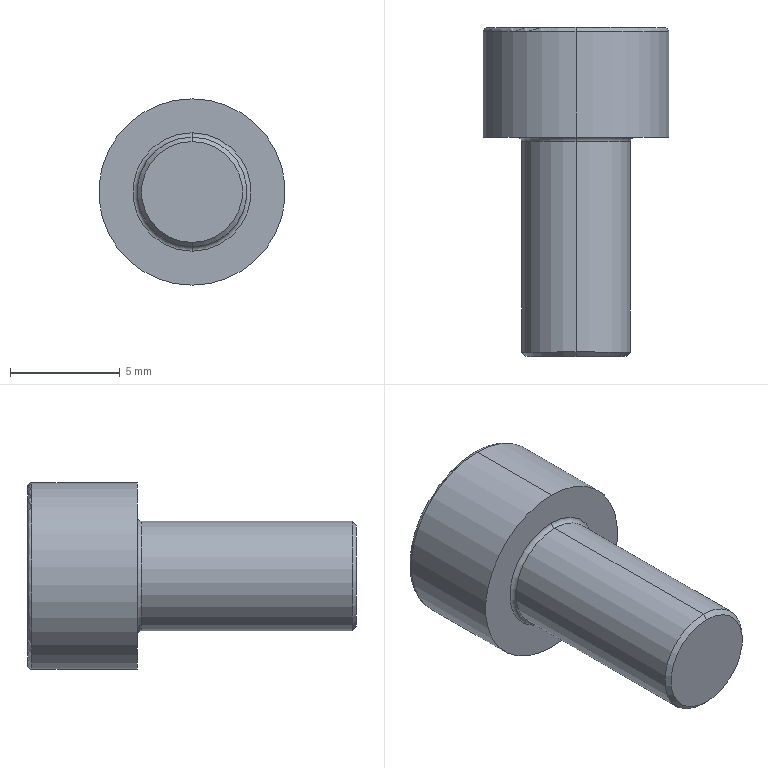Part | STEP file | 1 solid | 20 faces | box 8.5 x 15 x 8.5 mm | volume 445.038 mm3 | plane 10 | torus 4 | cylinder 4 | cone 2 | commonest cylinder face diameters 5 x2 8.5 x2
STEP:
#1=CARTESIAN_POINT('',(0.,-10.,-2.3));
#2=VERTEX_POINT('',#1);
#3=CARTESIAN_POINT('',(0.,-10.,2.3));
#4=VERTEX_POINT('',#3);
#5=CARTESIAN_POINT('',(0.,-10.,0.));
#6=DIRECTION('',(0.,-1.,0.));
#7=DIRECTION('',(0.,0.,-1.));
#8=AXIS2_PLACEMENT_3D('',#5,#6,#7);
#9=CIRCLE('',#8,2.3);
#10=EDGE_CURVE('',#2,#4,#9,.T.);
#11=ORIENTED_EDGE('',*,*,#10,.F.);
#12=CARTESIAN_POINT('',(0.,-9.8,-2.5));
#13=VERTEX_POINT('',#12);
#14=CARTESIAN_POINT('',(0.,-10.,-2.3));
#15=DIRECTION('',(0.,0.7071,-0.7071));
#16=VECTOR('',#15,1000.);
#17=LINE('',#14,#16);
#18=EDGE_CURVE('',#2,#13,#17,.T.);
#19=ORIENTED_EDGE('',*,*,#18,.T.);
#20=CARTESIAN_POINT('',(0.,-9.8,2.5));
#21=VERTEX_POINT('',#20);
#22=CARTESIAN_POINT('',(0.,-9.8,0.));
#23=DIRECTION('',(0.,1.,0.));
#24=DIRECTION('',(0.,0.,-1.));
#25=AXIS2_PLACEMENT_3D('',#22,#23,#24);
#26=CIRCLE('',#25,2.5);
#27=EDGE_CURVE('',#21,#13,#26,.T.);
#28=ORIENTED_EDGE('',*,*,#27,.F.);
#29=CARTESIAN_POINT('',(0.,-10.,2.3));
#30=DIRECTION('',(0.,0.7071,0.7071));
#31=VECTOR('',#30,1000.);
#32=LINE('',#29,#31);
#33=EDGE_CURVE('',#4,#21,#32,.T.);
#34=ORIENTED_EDGE('',*,*,#33,.F.);
#35=EDGE_LOOP('',(#11,#19,#28,#34));
#36=FACE_OUTER_BOUND('',#35,.T.);
#37=CARTESIAN_POINT('',(0.,-10.,0.));
#38=DIRECTION('',(0.,1.,0.));
#39=DIRECTION('',(0.,0.,1.));
#40=AXIS2_PLACEMENT_3D('',#37,#38,#39);
#41=CONICAL_SURFACE('',#40,2.3,0.7854);
#42=ADVANCED_FACE('',(#36),#41,.T.);
#43=CARTESIAN_POINT('',(0.,4.8,-4.25));
#44=VERTEX_POINT('',#43);
#45=CARTESIAN_POINT('',(0.,4.8,4.25));
#46=VERTEX_POINT('',#45);
#47=CARTESIAN_POINT('',(0.,4.8,0.));
#48=DIRECTION('',(0.,-1.,0.));
#49=DIRECTION('',(0.,0.,1.));
#50=AXIS2_PLACEMENT_3D('',#47,#48,#49);
#51=CIRCLE('',#50,4.25);
#52=EDGE_CURVE('',#44,#46,#51,.T.);
#53=ORIENTED_EDGE('',*,*,#52,.F.);
#54=CARTESIAN_POINT('',(0.,5.,-4.05));
#55=VERTEX_POINT('',#54);
#56=CARTESIAN_POINT('',(0.,4.8,-4.05));
#57=DIRECTION('',(1.,0.,0.));
#58=DIRECTION('',(0.,0.,-1.));
#59=AXIS2_PLACEMENT_3D('',#56,#57,#58);
#60=CIRCLE('',#59,0.2);
#61=EDGE_CURVE('',#44,#55,#60,.T.);
#62=ORIENTED_EDGE('',*,*,#61,.T.);
#63=CARTESIAN_POINT('',(0.,5.,4.05));
#64=VERTEX_POINT('',#63);
#65=CARTESIAN_POINT('',(0.,5.,0.));
#66=DIRECTION('',(0.,1.,0.));
#67=DIRECTION('',(0.,0.,1.));
#68=AXIS2_PLACEMENT_3D('',#65,#66,#67);
#69=CIRCLE('',#68,4.05);
#70=EDGE_CURVE('',#64,#55,#69,.T.);
#71=ORIENTED_EDGE('',*,*,#70,.F.);
#72=CARTESIAN_POINT('',(0.,4.8,4.05));
#73=DIRECTION('',(-1.,0.,0.));
#74=DIRECTION('',(0.,0.,1.));
#75=AXIS2_PLACEMENT_3D('',#72,#73,#74);
#76=CIRCLE('',#75,0.2);
#77=EDGE_CURVE('',#46,#64,#76,.T.);
#78=ORIENTED_EDGE('',*,*,#77,.F.);
#79=EDGE_LOOP('',(#53,#62,#71,#78));
#80=FACE_OUTER_BOUND('',#79,.T.);
#81=CARTESIAN_POINT('',(0.,4.8,0.));
#82=DIRECTION('',(0.,1.,0.));
#83=DIRECTION('',(0.,0.,1.));
#84=AXIS2_PLACEMENT_3D('',#81,#82,#83);
#85=TOROIDAL_SURFACE('',#84,4.05,0.2);
#86=ADVANCED_FACE('',(#80),#85,.T.);
#87=CARTESIAN_POINT('',(0.,-0.2,2.5));
#88=VERTEX_POINT('',#87);
#89=CARTESIAN_POINT('',(0.,-0.2,-2.5));
#90=VERTEX_POINT('',#89);
#91=CARTESIAN_POINT('',(0.,-0.2,0.));
#92=DIRECTION('',(0.,-1.,0.));
#93=DIRECTION('',(0.,0.,-1.));
#94=AXIS2_PLACEMENT_3D('',#91,#92,#93);
#95=CIRCLE('',#94,2.5);
#96=EDGE_CURVE('',#88,#90,#95,.T.);
#97=ORIENTED_EDGE('',*,*,#96,.F.);
#98=CARTESIAN_POINT('',(0.,0.,2.7));
#99=VERTEX_POINT('',#98);
#100=CARTESIAN_POINT('',(0.,-0.2,2.7));
#101=DIRECTION('',(1.,0.,0.));
#102=DIRECTION('',(0.,0.,-1.));
#103=AXIS2_PLACEMENT_3D('',#100,#101,#102);
#104=CIRCLE('',#103,0.2);
#105=EDGE_CURVE('',#88,#99,#104,.T.);
#106=ORIENTED_EDGE('',*,*,#105,.T.);
#107=CARTESIAN_POINT('',(0.,0.,-2.7));
#108=VERTEX_POINT('',#107);
#109=CARTESIAN_POINT('',(0.,0.,0.));
#110=DIRECTION('',(0.,1.,0.));
#111=DIRECTION('',(0.,0.,-1.));
#112=AXIS2_PLACEMENT_3D('',#109,#110,#111);
#113=CIRCLE('',#112,2.7);
#114=EDGE_CURVE('',#108,#99,#113,.T.);
#115=ORIENTED_EDGE('',*,*,#114,.F.);
#116=CARTESIAN_POINT('',(0.,-0.2,-2.7));
#117=DIRECTION('',(-1.,0.,0.));
#118=DIRECTION('',(0.,0.,1.));
#119=AXIS2_PLACEMENT_3D('',#116,#117,#118);
#120=CIRCLE('',#119,0.2);
#121=EDGE_CURVE('',#90,#108,#120,.T.);
#122=ORIENTED_EDGE('',*,*,#121,.F.);
#123=EDGE_LOOP('',(#97,#106,#115,#122));
#124=FACE_OUTER_BOUND('',#123,.T.);
#125=CARTESIAN_POINT('',(0.,-0.2,0.));
#126=DIRECTION('',(0.,-1.,0.));
#127=DIRECTION('',(0.,0.,-1.));
#128=AXIS2_PLACEMENT_3D('',#125,#126,#127);
#129=TOROIDAL_SURFACE('',#128,2.7,0.2);
#130=ADVANCED_FACE('',(#124),#129,.F.);
#131=CARTESIAN_POINT('',(0.,-0.2,0.));
#132=DIRECTION('',(0.,-1.,0.));
#133=DIRECTION('',(0.,0.,-1.));
#134=AXIS2_PLACEMENT_3D('',#131,#132,#133);
#135=CIRCLE('',#134,2.5);
#136=EDGE_CURVE('',#90,#88,#135,.T.);
#137=ORIENTED_EDGE('',*,*,#136,.T.);
#138=CARTESIAN_POINT('',(0.,0.,2.5));
#139=DIRECTION('',(0.,-1.,0.));
#140=VECTOR('',#139,1000.);
#141=LINE('',#138,#140);
#142=EDGE_CURVE('',#88,#21,#141,.T.);
#143=ORIENTED_EDGE('',*,*,#142,.T.);
#144=ORIENTED_EDGE('',*,*,#27,.T.);
#145=CARTESIAN_POINT('',(0.,0.,-2.5));
#146=DIRECTION('',(0.,-1.,0.));
#147=VECTOR('',#146,1000.);
#148=LINE('',#145,#147);
#149=EDGE_CURVE('',#90,#13,#148,.T.);
#150=ORIENTED_EDGE('',*,*,#149,.F.);
#151=EDGE_LOOP('',(#137,#143,#144,#150));
#152=FACE_OUTER_BOUND('',#151,.T.);
#153=CARTESIAN_POINT('',(0.,0.,0.));
#154=DIRECTION('',(0.,-1.,0.));
#155=DIRECTION('',(0.,0.,-1.));
#156=AXIS2_PLACEMENT_3D('',#153,#154,#155);
#157=CYLINDRICAL_SURFACE('',#156,2.5);
#158=ADVANCED_FACE('',(#152),#157,.T.);
#159=ORIENTED_EDGE('',*,*,#52,.T.);
#160=CARTESIAN_POINT('',(0.,0.,4.25));
#161=VERTEX_POINT('',#160);
#162=CARTESIAN_POINT('',(0.,0.,4.25));
#163=DIRECTION('',(0.,-1.,0.));
#164=VECTOR('',#163,1000.);
#165=LINE('',#162,#164);
#166=EDGE_CURVE('',#46,#161,#165,.T.);
#167=ORIENTED_EDGE('',*,*,#166,.T.);
#168=CARTESIAN_POINT('',(0.,0.,-4.25));
#169=VERTEX_POINT('',#168);
#170=CARTESIAN_POINT('',(0.,0.,0.));
#171=DIRECTION('',(0.,-1.,0.));
#172=DIRECTION('',(0.,0.,-1.));
#173=AXIS2_PLACEMENT_3D('',#170,#171,#172);
#174=CIRCLE('',#173,4.25);
#175=EDGE_CURVE('',#169,#161,#174,.T.);
#176=ORIENTED_EDGE('',*,*,#175,.F.);
#177=CARTESIAN_POINT('',(0.,0.,-4.25));
#178=DIRECTION('',(0.,-1.,0.));
#179=VECTOR('',#178,1000.);
#180=LINE('',#177,#179);
#181=EDGE_CURVE('',#44,#169,#180,.T.);
#182=ORIENTED_EDGE('',*,*,#181,.F.);
#183=EDGE_LOOP('',(#159,#167,#176,#182));
#184=FACE_OUTER_BOUND('',#183,.T.);
#185=CARTESIAN_POINT('',(0.,0.,0.));
#186=DIRECTION('',(0.,-1.,0.));
#187=DIRECTION('',(0.,0.,-1.));
#188=AXIS2_PLACEMENT_3D('',#185,#186,#187);
#189=CYLINDRICAL_SURFACE('',#188,4.25);
#190=ADVANCED_FACE('',(#184),#189,.T.);
#191=ORIENTED_EDGE('',*,*,#70,.T.);
#192=CARTESIAN_POINT('',(0.,5.,0.));
#193=DIRECTION('',(0.,1.,0.));
#194=DIRECTION('',(0.,0.,1.));
#195=AXIS2_PLACEMENT_3D('',#192,#193,#194);
#196=CIRCLE('',#195,4.05);
#197=EDGE_CURVE('',#55,#64,#196,.T.);
#198=ORIENTED_EDGE('',*,*,#197,.T.);
#199=EDGE_LOOP('',(#191,#198));
#200=FACE_OUTER_BOUND('',#199,.T.);
#201=CARTESIAN_POINT('',(0.,5.,-2.309));
#202=VERTEX_POINT('',#201);
#203=CARTESIAN_POINT('',(-2.,5.,-1.155));
#204=VERTEX_POINT('',#203);
#205=CARTESIAN_POINT('',(0.,5.,-2.309));
#206=DIRECTION('',(-0.866,0.,0.5));
#207=VECTOR('',#206,1000.);
#208=LINE('',#205,#207);
#209=EDGE_CURVE('',#202,#204,#208,.T.);
#210=ORIENTED_EDGE('',*,*,#209,.F.);
#211=CARTESIAN_POINT('',(2.,5.,-1.155));
#212=VERTEX_POINT('',#211);
#213=CARTESIAN_POINT('',(2.,5.,-1.155));
#214=DIRECTION('',(-0.866,0.,-0.5));
#215=VECTOR('',#214,1000.);
#216=LINE('',#213,#215);
#217=EDGE_CURVE('',#212,#202,#216,.T.);
#218=ORIENTED_EDGE('',*,*,#217,.F.);
#219=CARTESIAN_POINT('',(2.,5.,1.155));
#220=VERTEX_POINT('',#219);
#221=CARTESIAN_POINT('',(2.,5.,1.155));
#222=DIRECTION('',(0.,0.,-1.));
#223=VECTOR('',#222,1000.);
#224=LINE('',#221,#223);
#225=EDGE_CURVE('',#220,#212,#224,.T.);
#226=ORIENTED_EDGE('',*,*,#225,.F.);
#227=CARTESIAN_POINT('',(0.,5.,2.309));
#228=VERTEX_POINT('',#227);
#229=CARTESIAN_POINT('',(0.,5.,2.309));
#230=DIRECTION('',(0.866,0.,-0.5));
#231=VECTOR('',#230,1000.);
#232=LINE('',#229,#231);
#233=EDGE_CURVE('',#228,#220,#232,.T.);
#234=ORIENTED_EDGE('',*,*,#233,.F.);
#235=CARTESIAN_POINT('',(-2.,5.,1.155));
#236=VERTEX_POINT('',#235);
#237=CARTESIAN_POINT('',(-2.,5.,1.155));
#238=DIRECTION('',(0.866,0.,0.5));
#239=VECTOR('',#238,1000.);
#240=LINE('',#237,#239);
#241=EDGE_CURVE('',#236,#228,#240,.T.);
#242=ORIENTED_EDGE('',*,*,#241,.F.);
#243=CARTESIAN_POINT('',(-2.,5.,-1.155));
#244=DIRECTION('',(0.,0.,1.));
#245=VECTOR('',#244,1000.);
#246=LINE('',#243,#245);
#247=EDGE_CURVE('',#204,#236,#246,.T.);
#248=ORIENTED_EDGE('',*,*,#247,.F.);
#249=EDGE_LOOP('',(#210,#218,#226,#234,#242,#248));
#250=FACE_BOUND('',#249,.T.);
#251=CARTESIAN_POINT('',(0.,5.,0.));
#252=DIRECTION('',(0.,1.,0.));
#253=DIRECTION('',(0.,0.,1.));
#254=AXIS2_PLACEMENT_3D('',#251,#252,#253);
#255=PLANE('',#254);
#256=ADVANCED_FACE('',(#200,#250),#255,.T.);
#257=ORIENTED_EDGE('',*,*,#166,.F.);
#258=CARTESIAN_POINT('',(0.,4.8,0.));
#259=DIRECTION('',(0.,-1.,0.));
#260=DIRECTION('',(0.,0.,1.));
#261=AXIS2_PLACEMENT_3D('',#258,#259,#260);
#262=CIRCLE('',#261,4.25);
#263=EDGE_CURVE('',#46,#44,#262,.T.);
#264=ORIENTED_EDGE('',*,*,#263,.T.);
#265=ORIENTED_EDGE('',*,*,#181,.T.);
#266=CARTESIAN_POINT('',(0.,0.,0.));
#267=DIRECTION('',(0.,-1.,0.));
#268=DIRECTION('',(0.,0.,-1.));
#269=AXIS2_PLACEMENT_3D('',#266,#267,#268);
#270=CIRCLE('',#269,4.25);
#271=EDGE_CURVE('',#161,#169,#270,.T.);
#272=ORIENTED_EDGE('',*,*,#271,.F.);
#273=EDGE_LOOP('',(#257,#264,#265,#272));
#274=FACE_OUTER_BOUND('',#273,.T.);
#275=CARTESIAN_POINT('',(0.,0.,0.));
#276=DIRECTION('',(0.,-1.,0.));
#277=DIRECTION('',(0.,0.,-1.));
#278=AXIS2_PLACEMENT_3D('',#275,#276,#277);
#279=CYLINDRICAL_SURFACE('',#278,4.25);
#280=ADVANCED_FACE('',(#274),#279,.T.);
#281=ORIENTED_EDGE('',*,*,#114,.T.);
#282=CARTESIAN_POINT('',(0.,0.,0.));
#283=DIRECTION('',(0.,1.,0.));
#284=DIRECTION('',(0.,0.,-1.));
#285=AXIS2_PLACEMENT_3D('',#282,#283,#284);
#286=CIRCLE('',#285,2.7);
#287=EDGE_CURVE('',#99,#108,#286,.T.);
#288=ORIENTED_EDGE('',*,*,#287,.T.);
#289=EDGE_LOOP('',(#281,#288));
#290=FACE_BOUND('',#289,.T.);
#291=ORIENTED_EDGE('',*,*,#175,.T.);
#292=ORIENTED_EDGE('',*,*,#271,.T.);
#293=EDGE_LOOP('',(#291,#292));
#294=FACE_OUTER_BOUND('',#293,.T.);
#295=CARTESIAN_POINT('',(4.25,0.,0.));
#296=DIRECTION('',(0.,-1.,0.));
#297=DIRECTION('',(0.,0.,-1.));
#298=AXIS2_PLACEMENT_3D('',#295,#296,#297);
#299=PLANE('',#298);
#300=ADVANCED_FACE('',(#290,#294),#299,.T.);
#301=ORIENTED_EDGE('',*,*,#142,.F.);
#302=ORIENTED_EDGE('',*,*,#96,.T.);
#303=ORIENTED_EDGE('',*,*,#149,.T.);
#304=CARTESIAN_POINT('',(0.,-9.8,0.));
#305=DIRECTION('',(0.,1.,0.));
#306=DIRECTION('',(0.,0.,-1.));
#307=AXIS2_PLACEMENT_3D('',#304,#305,#306);
#308=CIRCLE('',#307,2.5);
#309=EDGE_CURVE('',#13,#21,#308,.T.);
#310=ORIENTED_EDGE('',*,*,#309,.T.);
#311=EDGE_LOOP('',(#301,#302,#303,#310));
#312=FACE_OUTER_BOUND('',#311,.T.);
#313=CARTESIAN_POINT('',(0.,0.,0.));
#314=DIRECTION('',(0.,-1.,0.));
#315=DIRECTION('',(0.,0.,-1.));
#316=AXIS2_PLACEMENT_3D('',#313,#314,#315);
#317=CYLINDRICAL_SURFACE('',#316,2.5);
#318=ADVANCED_FACE('',(#312),#317,.T.);
#319=CARTESIAN_POINT('',(0.,-10.,0.));
#320=DIRECTION('',(0.,-1.,0.));
#321=DIRECTION('',(0.,0.,-1.));
#322=AXIS2_PLACEMENT_3D('',#319,#320,#321);
#323=CIRCLE('',#322,2.3);
#324=EDGE_CURVE('',#4,#2,#323,.T.);
#325=ORIENTED_EDGE('',*,*,#324,.T.);
#326=ORIENTED_EDGE('',*,*,#10,.T.);
#327=EDGE_LOOP('',(#325,#326));
#328=FACE_OUTER_BOUND('',#327,.T.);
#329=CARTESIAN_POINT('',(2.5,-10.,0.));
#330=DIRECTION('',(0.,-1.,0.));
#331=DIRECTION('',(0.,0.,-1.));
#332=AXIS2_PLACEMENT_3D('',#329,#330,#331);
#333=PLANE('',#332);
#334=ADVANCED_FACE('',(#328),#333,.T.);
#335=ORIENTED_EDGE('',*,*,#209,.T.);
#336=CARTESIAN_POINT('',(-2.,2.5,-1.155));
#337=VERTEX_POINT('',#336);
#338=CARTESIAN_POINT('',(-2.,2.5,-1.155));
#339=DIRECTION('',(0.,1.,0.));
#340=VECTOR('',#339,1000.);
#341=LINE('',#338,#340);
#342=EDGE_CURVE('',#337,#204,#341,.T.);
#343=ORIENTED_EDGE('',*,*,#342,.F.);
#344=CARTESIAN_POINT('',(0.,2.5,-2.309));
#345=VERTEX_POINT('',#344);
#346=CARTESIAN_POINT('',(0.,2.5,-2.309));
#347=DIRECTION('',(-0.866,0.,0.5));
#348=VECTOR('',#347,1000.);
#349=LINE('',#346,#348);
#350=EDGE_CURVE('',#345,#337,#349,.T.);
#351=ORIENTED_EDGE('',*,*,#350,.F.);
#352=CARTESIAN_POINT('',(0.,2.5,-2.309));
#353=DIRECTION('',(0.,1.,0.));
#354=VECTOR('',#353,1000.);
#355=LINE('',#352,#354);
#356=EDGE_CURVE('',#345,#202,#355,.T.);
#357=ORIENTED_EDGE('',*,*,#356,.T.);
#358=EDGE_LOOP('',(#335,#343,#351,#357));
#359=FACE_OUTER_BOUND('',#358,.T.);
#360=CARTESIAN_POINT('',(0.,2.5,-2.309));
#361=DIRECTION('',(-0.5,0.,-0.866));
#362=DIRECTION('',(-0.866,0.,0.5));
#363=AXIS2_PLACEMENT_3D('',#360,#361,#362);
#364=PLANE('',#363);
#365=ADVANCED_FACE('',(#359),#364,.F.);
#366=ORIENTED_EDGE('',*,*,#217,.T.);
#367=ORIENTED_EDGE('',*,*,#356,.F.);
#368=CARTESIAN_POINT('',(2.,2.5,-1.155));
#369=VERTEX_POINT('',#368);
#370=CARTESIAN_POINT('',(2.,2.5,-1.155));
#371=DIRECTION('',(-0.866,0.,-0.5));
#372=VECTOR('',#371,1000.);
#373=LINE('',#370,#372);
#374=EDGE_CURVE('',#369,#345,#373,.T.);
#375=ORIENTED_EDGE('',*,*,#374,.F.);
#376=CARTESIAN_POINT('',(2.,2.5,-1.155));
#377=DIRECTION('',(0.,1.,0.));
#378=VECTOR('',#377,1000.);
#379=LINE('',#376,#378);
#380=EDGE_CURVE('',#369,#212,#379,.T.);
#381=ORIENTED_EDGE('',*,*,#380,.T.);
#382=EDGE_LOOP('',(#366,#367,#375,#381));
#383=FACE_OUTER_BOUND('',#382,.T.);
#384=CARTESIAN_POINT('',(2.,2.5,-1.155));
#385=DIRECTION('',(0.5,0.,-0.866));
#386=DIRECTION('',(-0.866,0.,-0.5));
#387=AXIS2_PLACEMENT_3D('',#384,#385,#386);
#388=PLANE('',#387);
#389=ADVANCED_FACE('',(#383),#388,.F.);
#390=ORIENTED_EDGE('',*,*,#225,.T.);
#391=ORIENTED_EDGE('',*,*,#380,.F.);
#392=CARTESIAN_POINT('',(2.,2.5,1.155));
#393=VERTEX_POINT('',#392);
#394=CARTESIAN_POINT('',(2.,2.5,1.155));
#395=DIRECTION('',(0.,0.,-1.));
#396=VECTOR('',#395,1000.);
#397=LINE('',#394,#396);
#398=EDGE_CURVE('',#393,#369,#397,.T.);
#399=ORIENTED_EDGE('',*,*,#398,.F.);
#400=CARTESIAN_POINT('',(2.,2.5,1.155));
#401=DIRECTION('',(0.,1.,0.));
#402=VECTOR('',#401,1000.);
#403=LINE('',#400,#402);
#404=EDGE_CURVE('',#393,#220,#403,.T.);
#405=ORIENTED_EDGE('',*,*,#404,.T.);
#406=EDGE_LOOP('',(#390,#391,#399,#405));
#407=FACE_OUTER_BOUND('',#406,.T.);
#408=CARTESIAN_POINT('',(2.,2.5,1.155));
#409=DIRECTION('',(1.,0.,0.));
#410=DIRECTION('',(0.,0.,-1.));
#411=AXIS2_PLACEMENT_3D('',#408,#409,#410);
#412=PLANE('',#411);
#413=ADVANCED_FACE('',(#407),#412,.F.);
#414=ORIENTED_EDGE('',*,*,#233,.T.);
#415=ORIENTED_EDGE('',*,*,#404,.F.);
#416=CARTESIAN_POINT('',(0.,2.5,2.309));
#417=VERTEX_POINT('',#416);
#418=CARTESIAN_POINT('',(0.,2.5,2.309));
#419=DIRECTION('',(0.866,0.,-0.5));
#420=VECTOR('',#419,1000.);
#421=LINE('',#418,#420);
#422=EDGE_CURVE('',#417,#393,#421,.T.);
#423=ORIENTED_EDGE('',*,*,#422,.F.);
#424=CARTESIAN_POINT('',(0.,2.5,2.309));
#425=DIRECTION('',(0.,1.,0.));
#426=VECTOR('',#425,1000.);
#427=LINE('',#424,#426);
#428=EDGE_CURVE('',#417,#228,#427,.T.);
#429=ORIENTED_EDGE('',*,*,#428,.T.);
#430=EDGE_LOOP('',(#414,#415,#423,#429));
#431=FACE_OUTER_BOUND('',#430,.T.);
#432=CARTESIAN_POINT('',(0.,2.5,2.309));
#433=DIRECTION('',(0.5,0.,0.866));
#434=DIRECTION('',(0.866,0.,-0.5));
#435=AXIS2_PLACEMENT_3D('',#432,#433,#434);
#436=PLANE('',#435);
#437=ADVANCED_FACE('',(#431),#436,.F.);
#438=ORIENTED_EDGE('',*,*,#241,.T.);
#439=ORIENTED_EDGE('',*,*,#428,.F.);
#440=CARTESIAN_POINT('',(-2.,2.5,1.155));
#441=VERTEX_POINT('',#440);
#442=CARTESIAN_POINT('',(-2.,2.5,1.155));
#443=DIRECTION('',(0.866,0.,0.5));
#444=VECTOR('',#443,1000.);
#445=LINE('',#442,#444);
#446=EDGE_CURVE('',#441,#417,#445,.T.);
#447=ORIENTED_EDGE('',*,*,#446,.F.);
#448=CARTESIAN_POINT('',(-2.,2.5,1.155));
#449=DIRECTION('',(0.,1.,0.));
#450=VECTOR('',#449,1000.);
#451=LINE('',#448,#450);
#452=EDGE_CURVE('',#441,#236,#451,.T.);
#453=ORIENTED_EDGE('',*,*,#452,.T.);
#454=EDGE_LOOP('',(#438,#439,#447,#453));
#455=FACE_OUTER_BOUND('',#454,.T.);
#456=CARTESIAN_POINT('',(-2.,2.5,1.155));
#457=DIRECTION('',(-0.5,0.,0.866));
#458=DIRECTION('',(0.866,0.,0.5));
#459=AXIS2_PLACEMENT_3D('',#456,#457,#458);
#460=PLANE('',#459);
#461=ADVANCED_FACE('',(#455),#460,.F.);
#462=ORIENTED_EDGE('',*,*,#247,.T.);
#463=ORIENTED_EDGE('',*,*,#452,.F.);
#464=CARTESIAN_POINT('',(-2.,2.5,-1.155));
#465=DIRECTION('',(0.,0.,1.));
#466=VECTOR('',#465,1000.);
#467=LINE('',#464,#466);
#468=EDGE_CURVE('',#337,#441,#467,.T.);
#469=ORIENTED_EDGE('',*,*,#468,.F.);
#470=ORIENTED_EDGE('',*,*,#342,.T.);
#471=EDGE_LOOP('',(#462,#463,#469,#470));
#472=FACE_OUTER_BOUND('',#471,.T.);
#473=CARTESIAN_POINT('',(-2.,2.5,-1.155));
#474=DIRECTION('',(-1.,0.,0.));
#475=DIRECTION('',(0.,0.,1.));
#476=AXIS2_PLACEMENT_3D('',#473,#474,#475);
#477=PLANE('',#476);
#478=ADVANCED_FACE('',(#472),#477,.F.);
#479=ORIENTED_EDGE('',*,*,#350,.T.);
#480=ORIENTED_EDGE('',*,*,#468,.T.);
#481=ORIENTED_EDGE('',*,*,#446,.T.);
#482=ORIENTED_EDGE('',*,*,#422,.T.);
#483=ORIENTED_EDGE('',*,*,#398,.T.);
#484=ORIENTED_EDGE('',*,*,#374,.T.);
#485=EDGE_LOOP('',(#479,#480,#481,#482,#483,#484));
#486=FACE_OUTER_BOUND('',#485,.T.);
#487=CARTESIAN_POINT('',(0.,2.5,0.));
#488=DIRECTION('',(0.,1.,0.));
#489=DIRECTION('',(0.,0.,1.));
#490=AXIS2_PLACEMENT_3D('',#487,#488,#489);
#491=PLANE('',#490);
#492=ADVANCED_FACE('',(#486),#491,.T.);
#493=ORIENTED_EDGE('',*,*,#105,.F.);
#494=ORIENTED_EDGE('',*,*,#136,.F.);
#495=ORIENTED_EDGE('',*,*,#121,.T.);
#496=ORIENTED_EDGE('',*,*,#287,.F.);
#497=EDGE_LOOP('',(#493,#494,#495,#496));
#498=FACE_OUTER_BOUND('',#497,.T.);
#499=CARTESIAN_POINT('',(0.,-0.2,0.));
#500=DIRECTION('',(0.,-1.,0.));
#501=DIRECTION('',(0.,0.,-1.));
#502=AXIS2_PLACEMENT_3D('',#499,#500,#501);
#503=TOROIDAL_SURFACE('',#502,2.7,0.2);
#504=ADVANCED_FACE('',(#498),#503,.F.);
#505=ORIENTED_EDGE('',*,*,#61,.F.);
#506=ORIENTED_EDGE('',*,*,#263,.F.);
#507=ORIENTED_EDGE('',*,*,#77,.T.);
#508=ORIENTED_EDGE('',*,*,#197,.F.);
#509=EDGE_LOOP('',(#505,#506,#507,#508));
#510=FACE_OUTER_BOUND('',#509,.T.);
#511=CARTESIAN_POINT('',(0.,4.8,0.));
#512=DIRECTION('',(0.,1.,0.));
#513=DIRECTION('',(0.,0.,1.));
#514=AXIS2_PLACEMENT_3D('',#511,#512,#513);
#515=TOROIDAL_SURFACE('',#514,4.05,0.2);
#516=ADVANCED_FACE('',(#510),#515,.T.);
#517=ORIENTED_EDGE('',*,*,#18,.F.);
#518=ORIENTED_EDGE('',*,*,#324,.F.);
#519=ORIENTED_EDGE('',*,*,#33,.T.);
#520=ORIENTED_EDGE('',*,*,#309,.F.);
#521=EDGE_LOOP('',(#517,#518,#519,#520));
#522=FACE_OUTER_BOUND('',#521,.T.);
#523=CARTESIAN_POINT('',(0.,-10.,0.));
#524=DIRECTION('',(0.,1.,0.));
#525=DIRECTION('',(0.,0.,1.));
#526=AXIS2_PLACEMENT_3D('',#523,#524,#525);
#527=CONICAL_SURFACE('',#526,2.3,0.7854);
#528=ADVANCED_FACE('',(#522),#527,.T.);
#529=CLOSED_SHELL('',(#42,#86,#130,#158,#190,#256,#280,#300,#318,#334,#365,#389,#413,#437,#461,#478,#492,#504,#516,#528));
#530=MANIFOLD_SOLID_BREP('',#529);
#531=CARTESIAN_POINT('',(0.,0.,0.));
#532=DIRECTION('',(0.,0.,1.));
#533=DIRECTION('',(1.,0.,0.));
#534=AXIS2_PLACEMENT_3D('',#531,#532,#533);
#535=(LENGTH_UNIT()NAMED_UNIT(*)SI_UNIT(.MILLI.,.METRE.));
#536=UNCERTAINTY_MEASURE_WITH_UNIT(LENGTH_MEASURE(0.00001),#535,'','');
#537=(NAMED_UNIT(*)PLANE_ANGLE_UNIT()SI_UNIT($,.RADIAN.));
#538=(NAMED_UNIT(*)SI_UNIT($,.STERADIAN.)SOLID_ANGLE_UNIT());
#539=(GEOMETRIC_REPRESENTATION_CONTEXT(3)GLOBAL_UNCERTAINTY_ASSIGNED_CONTEXT((#536))GLOBAL_UNIT_ASSIGNED_CONTEXT((#535,#537,#538))REPRESENTATION_CONTEXT('',''));
#540=ADVANCED_BREP_SHAPE_REPRESENTATION('',(#530,#534),#539);